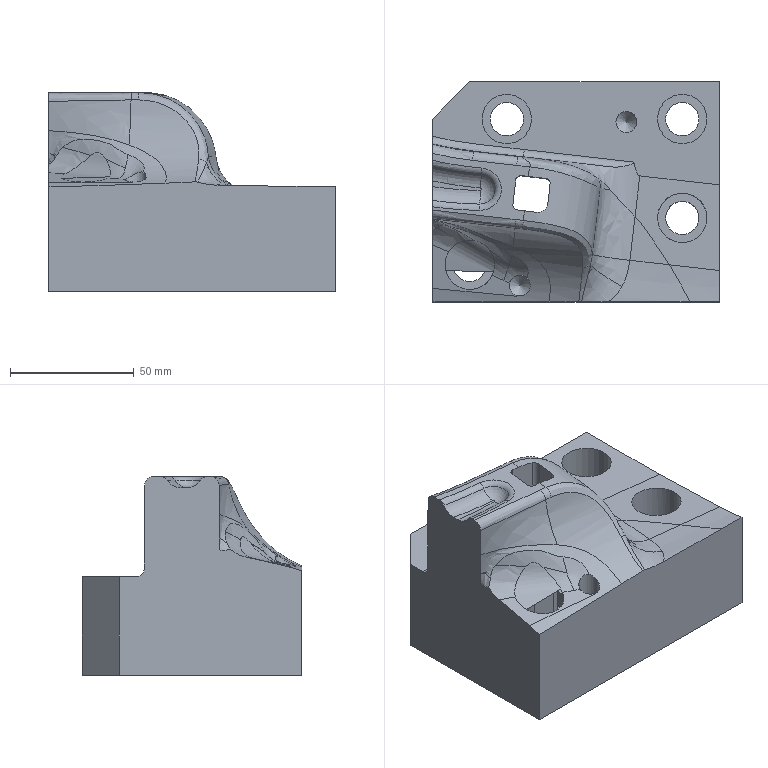Part | NX | features 23 2 | 1 solid | 97 faces | box 116 x 89 x 80.425 mm | volume 446580 mm3 | plane 34 | cylinder 28 | spline 26 | torus 7 | cone 2 | commonest cylinder face diameters 8 x5 20 x5 13.5 x4 15 x4 4 x3 7 x2